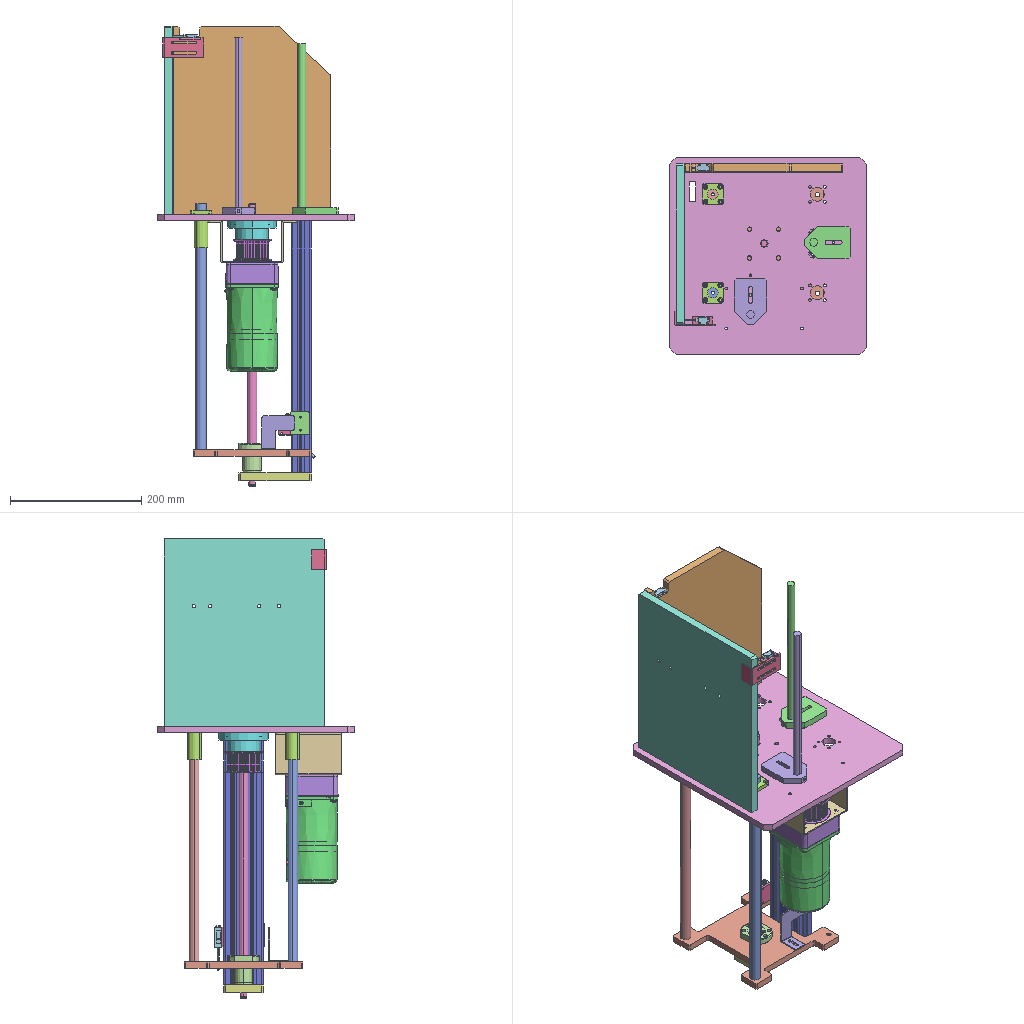Assembly | SolidWorks | 35 different items | 42 placed | box 300 x 300 x 701 mm
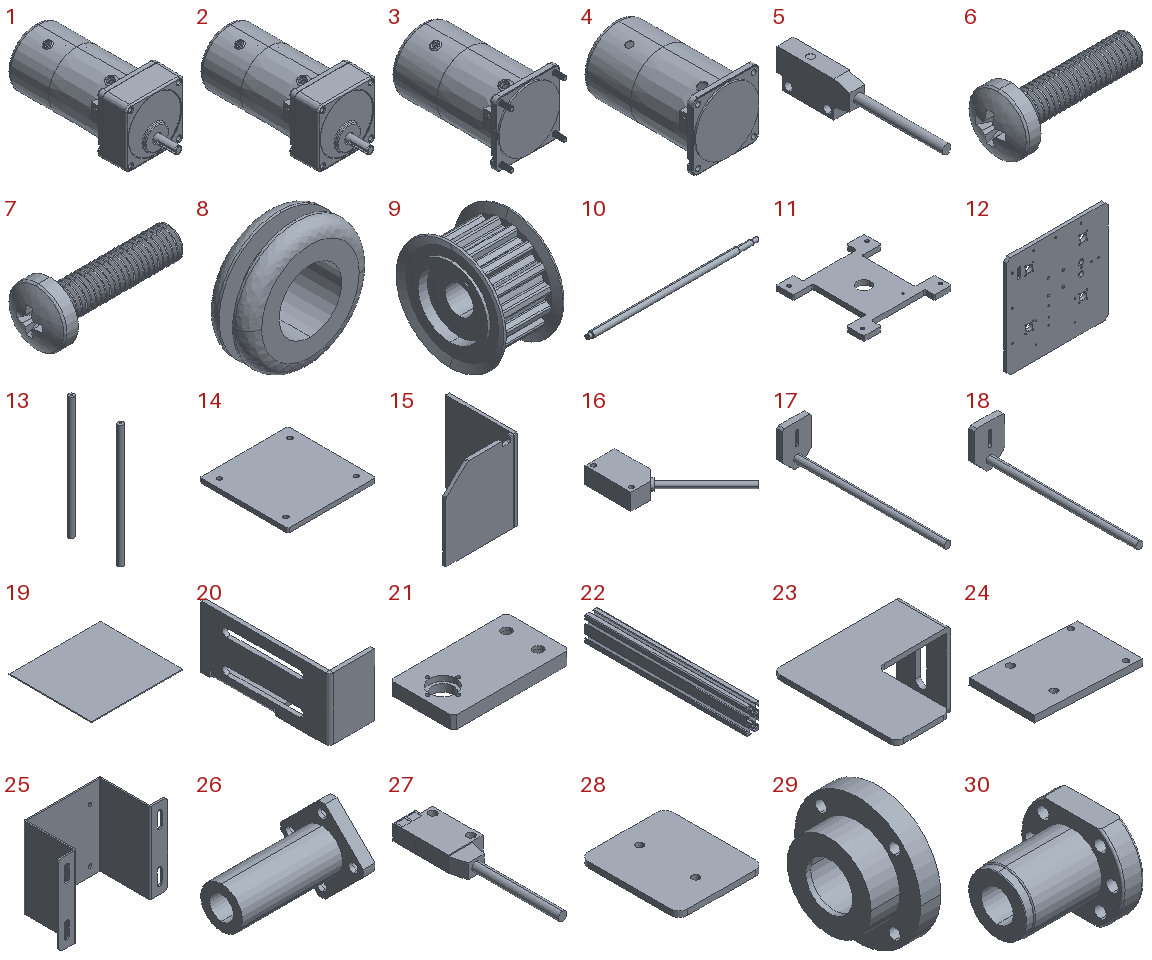Parts list (item | name | quantity | parent item | size | volume | features):
1 | (subassembly) | x1 | - | 81.315 x 196.821 x 80 mm | 357244 mm3 | -
2 | (subassembly) | x1 | - | 81.315 x 196.821 x 80 mm | 357244 mm3 | -
3 | (subassembly) | x1 | - | 81.301 x 146.321 x 79.972 mm | 169247 mm3 | -
4 | (subassembly) | x1 | in 3 | 79.972 x 134.7 x 79.972 mm | 165976 mm3 | -
5 | (subassembly) | x1 | - | 4.5 x 45.5 x 10 mm | 892.741 mm3 | -
6 | - | x1 | in 3 | 19.021 x 8 x 8 mm | 284.545 mm3 | features BaseBody 1
7 | - | x4 | in 3 | 23.632 x 9.5 x 9.5 mm | 537.774 mm3 | features BaseBody 1
8 | - | x1 | in 3 | 11.1 x 4 x 11.1 mm | 210.744 mm3 | features BaseBody 1
9 | - | x2 | - | 32 x 58 x 58 mm | 40036 mm3 | features Revolution 4, ICE 2, CirPattern 1, RefAxis 1
10 | - | x1 | - | 430 x 15 x 15 mm | 71115 mm3 | features Revolution 8, RevCut 7, ICE 5, RefAxis 3, Fillet 2
11 | - | x1 | - | 180 x 180 x 10 mm | 182649 mm3 | features HoleWzd 2, Chamfer 1, Cut 1, Extrusion 1, Fillet 1
12 | - | x1 | - | 300 x 10 x 300 mm | 864543 mm3 | features HoleWzd 6, Cut 3, Chamfer 1, Extrusion 1
13 | - | x1 | - | 16 x 166 x 375 mm | 136070 mm3 | features Extrusion 1, HoleWzd 1
14 | - | x1 | - | 200 x 200 x 10 mm | 397621 mm3 | features Chamfer 1, Extrusion 1, HoleWzd 1
15 | - | x2 | - | 254 x 245 x 287 mm | 1625619 mm3 | features Cut 3, Fillet 3, HoleWzd 3, Chamfer 2, Extrusion 1
16 | - | x1 | - | 54.507 x 67.507 x 11.2 mm | 7170 mm3 | features BaseBody 3
17 | - | x1 | - | 50 x 270 x 70 mm | 58386 mm3 | features ICE 2, Chamfer 1, Extrusion 1, HoleWzd 1
18 | - | x1 | - | 50 x 260 x 70 mm | 57256 mm3 | features ICE 3, Chamfer 1, Extrusion 1, HoleWzd 1
19 | - | x1 | - | 220 x 200 x 2 mm | 88000 mm3 | features Extrusion 1
20 | - | x1 | - | 22 x 62 x 30 mm | 4961 mm3 | features EdgeFlange 1, FlatPattern 1, ICE 1, SMBaseFlange 1, SheetMetal 1
21 | - | x1 | - | 110 x 60 x 12 mm | 70357 mm3 | features Cut 2, HoleWzd 2, Chamfer 1, Extrusion 1
22 | - | x1 | - | 30 x 384 x 60 mm | 244841 mm3 | features 3DProfileFeature 2, HoleWzd 2, WeldMemberFeat 1, WeldmentFeature 1
23 | - | x1 | - | 52 x 50 x 32 mm | 4399 mm3 | features Fillet 2, Cut 1, FlatPattern 1, ICE 1, SMBaseFlange 1, SheetMetal 1
24 | - | x1 | - | 50.086 x 30 x 5.375 mm | 4419 mm3 | features HoleWzd 2, Extrusion 1
25 | - | x1 | - | 135 x 64 x 100 mm | 49813 mm3 | features Cut 1, Fillet 1, FlatPattern 1, HoleWzd 1, ICE 1, SMBaseFlange 1, SheetMetal 1
26 | - | x2 | - | 57 x 42 x 42 mm | 16451 mm3 | features HoleWzd 2, ICE 2, CirPattern 1, Extrusion 1
27 | - | x2 | in 5 | 10 x 45.5 x 4.5 mm | 892.741 mm3 | features BaseBody 1
28 | - | x1 | - | 30 x 35 x 2 mm | 2065 mm3 | features Extrusion 1, Fillet 1, HoleWzd 1
29 | - | x1 | - | 29 x 75 x 75 mm | 54196 mm3 | features HoleWzd 2, Chamfer 1, Revolution 1
30 | - | x1 | - | 45 x 48 x 40 mm | 28053 mm3 | features ICE 3, RefAxis 3, HoleWzd 2, Revolution 2, CirPattern 1
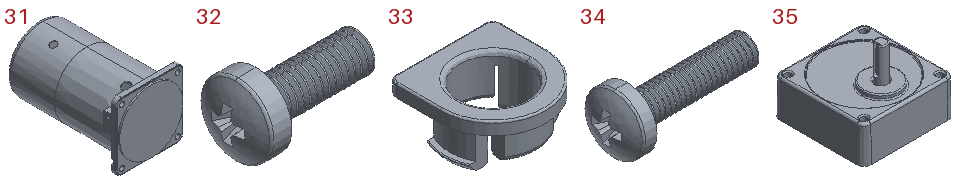31 | - | x1 | in 4 | 79.972 x 134.7 x 79.972 mm | 165976 mm3 | features BaseBody 1
32 | - | x1 | in 3 | 10.354 x 5.6 x 5.6 mm | 94.439 mm3 | features BaseBody 1
33 | - | x1 | in 3 | 12.5 x 12.5 x 6 mm | 243.257 mm3 | features BaseBody 1
34 | - | x1 | in 3 | 19.021 x 8 x 8 mm | 284.545 mm3 | features BaseBody 1
35 | - | x1 | - | 80 x 80 x 64 mm | 187976 mm3 | features BaseBody 1
Mates (type | each side: item.copy, entity, surface, feature):
Concentric | 13.1 face cylinder Boss-Extrude1 | 26.1 face cylinder Boss-Extrude1
DistanceDim | 26.1 face plane Boss-Extrude1 | 13.1 face plane Boss-Extrude1
Concentric | 13.1 face cylinder Boss-Extrude1 | 26.2 face cylinder Boss-Extrude1
DistanceDim | 26.2 face plane Boss-Extrude1 | 13.1 face plane Boss-Extrude1
DistanceDim | 12.1 face plane Boss-Extrude1 | 26.1 face plane Cut-Extrude1
DistanceDim | 26.1 face plane Cut-Extrude1 | 12.1 face plane Boss-Extrude1
Coincident | 12.1 face plane Boss-Extrude1 | 26.2 face plane Boss-Extrude2
Parallel | 12.1 face plane Boss-Extrude1 | 26.2 face plane Cut-Extrude1
Coincident | 15.1 face plane Boss-Extrude1 | 20.1 face plane Base-Flange1 | 2 times
Coincident | 15.1 face plane Cut-Extrude1 | 20.1 face plane Edge-Flange1
Coincident | 15.1 face plane Cut-Extrude1 | 27.1 face plane Input1
Parallel | 15.1 face plane Boss-Extrude1 | 27.1 face plane Input1
Coincident | 15.1 face plane Boss-Extrude1 | 27.1 face plane Input1
Coincident | 12.1 face plane Boss-Extrude1 | 17.1 face plane Boss-Extrude1
Coincident | 12.1 face plane Boss-Extrude1 | 18.1 face plane Boss-Extrude1
DistanceDim | 18.1 face plane Boss-Extrude1 | 12.1 face plane Boss-Extrude1
Coincident | 20.1 face plane Edge-Flange1 | 27.2 face plane Input1
Parallel | 20.1 face plane Base-Flange1 | 27.2 face plane Input1
DistanceDim | 27.2 face plane Input1 | 20.1 face plane Edge-Flange1
Coincident | 27.1 face plane Input1 | 27.2 face plane Input1
Coincident | 12.1 face plane Boss-Extrude1 | 22.1 face plane Aluminium profile 30 X 60 X R2(1) | 2 times
Coincident | 21.1 face plane Boss-Extrude1 | 22.1 face plane Aluminium profile 30 X 60 X R2(1)
Width | 11.1 face plane Boss-Extrude1 | 11.1 face plane Boss-Extrude1 | 22.1 face plane Aluminium profile 30 X 60 X R2(1) | 22.1 face plane Aluminium profile 30 X 60 X R2(1)
Coincident | 11.1 face plane Boss-Extrude1 | 30.1 face plane Revolve1
Concentric | 11.1 face cylinder Cut-Extrude1 | 30.1 face cylinder Revolve1
Parallel | 11.1 face plane Boss-Extrude1 | 30.1 face plane Cut-Extrude1
Concentric | 10.1 face cylinder Revolve1 | 21.1 face cylinder Cut-Extrude1
Concentric | 10.1 face cylinder Revolve1 | 9.1 face cylinder Revolve5
Coincident | 10.1 axis | 30.1 axis
Coincident | 10.1 plane | 30.1 plane
Coincident | 12.1 face plane Cut-Extrude1 | 29.1 edge
Concentric | 10.1 face cylinder Revolve1 | 29.1 face cylinder Revolve1
Coincident | 12.1 face plane Boss-Extrude1 | 25.1 face plane Base-Flange1
DistanceDim | 25.1 face plane Base-Flange1 | 12.1 face plane Boss-Extrude1
Concentric | 35.1 face cylinder Input1 | 25.1 face cylinder Cut-Extrude1
Coincident | 35.1 face plane Input1 | 25.1 face plane Base-Flange1
Coincident | 11.1 face plane Boss-Extrude1 | 23.1 face plane Base-Flange1
Parallel | 11.1 face plane Boss-Extrude1 | 23.1 face plane Base-Flange1
DistanceDim | 23.1 face plane Cut-Extrude1 | 11.1 face plane Boss-Extrude1
Coincident | 22.1 face plane Aluminium profile 30 X 60 X R2(1) | 28.1 face plane Boss-Extrude1
DistanceDim | 24.1 face plane Boss-Extrude1 | 21.1 face plane Boss-Extrude1
Coincident | 22.1 face plane Aluminium profile 30 X 60 X R2(1) | 24.1 face plane Boss-Extrude1 | 2 times
Coincident | 24.1 face plane Boss-Extrude1 | 16.1 face plane Input1 | 2 times
DistanceDim | 16.1 face plane Input1 | 24.1 face plane Boss-Extrude1
Concentric | 35.1 face cylinder Input1 | 9.2 face cylinder Revolve5
DistanceDim | 35.1 face plane Input1 | 9.2 face plane Revolve1